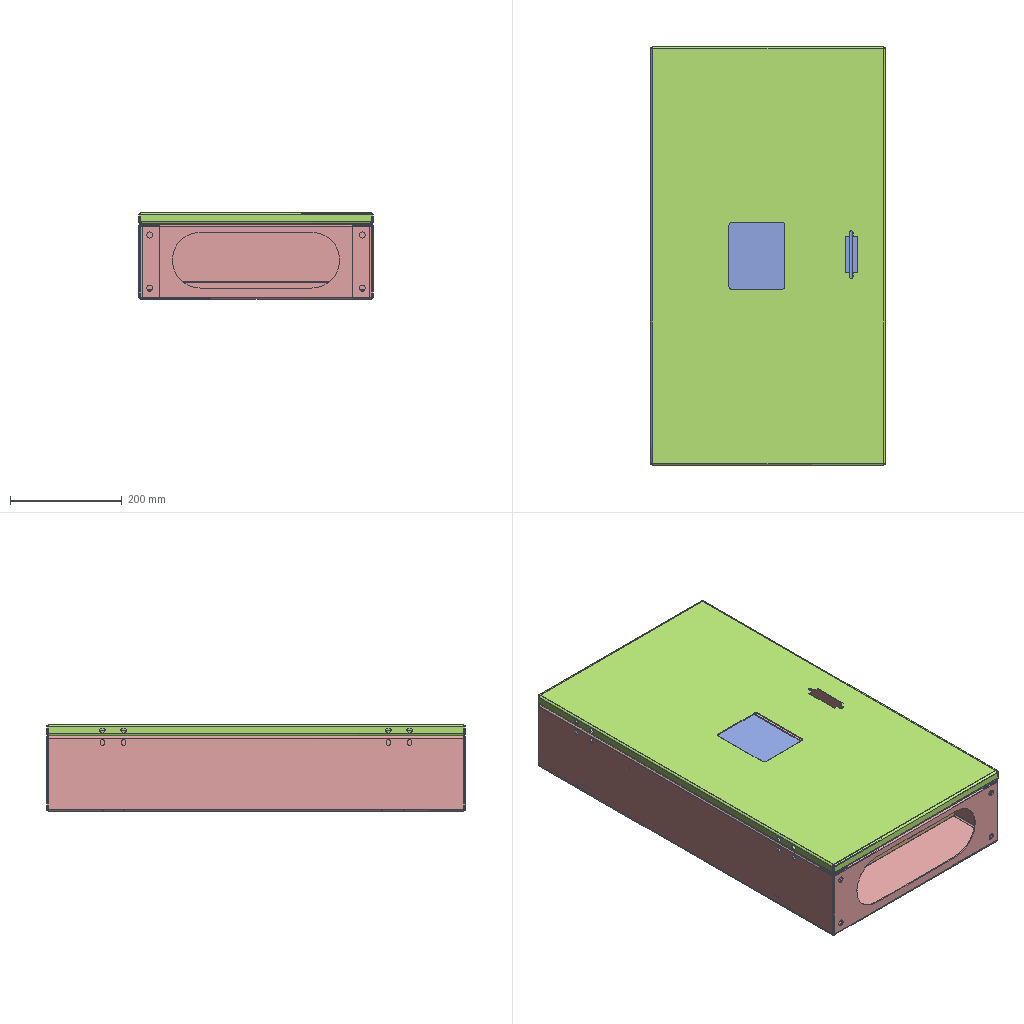Assembly | SolidWorks | 6 different items | 9 placed | box 420 x 750 x 155 mm
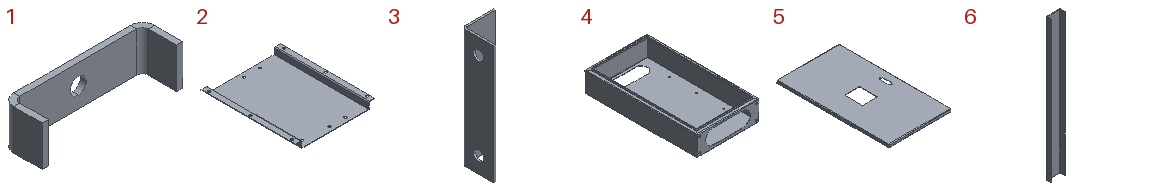Parts list (item | quantity | size | volume | features):
1 | x2 | 35 x 10 x 10 mm | 732.179 mm3 | features FlatPattern 1, ICE 1, SMBaseFlange 1, SheetMetal 1
2 | x1 | 350 x 415 x 30 mm | 330826 mm3 | features EdgeFlange 2, ICE 2, FlatPattern 1, SMBaseFlange 1, SheetMetal 1
3 | x2 | 35 x 35 x 130 mm | 16965 mm3 | features FlatPattern 1, ICE 1, SMBaseFlange 1, SheetMetal 1
4 | x1 | 420 x 750 x 145 mm | 1270936 mm3 | features ICE 5, EdgeFlange 3, FlatPattern 1, SMBaseFlange 1, SheetMetal 1
5 | x1 | 420 x 750 x 20 mm | 745969 mm3 | features ICE 3, EdgeFlange 2, FlatPattern 1, SMBaseFlange 1, SheetMetal 1
6 | x2 | 40 x 15 x 416 mm | 40603 mm3 | features FlatPattern 1, SMBaseFlange 1, SheetMetal 1
Mates (type | each side: item.copy, entity, surface, feature):
Coincident | 4.1 face plane Base-Flange1 | 2.1 face plane Edge-Flange2
Concentric | 4.1 face cylinder Cut-Extrude1 | 2.1 face cylinder Cut-Extrude2 | 2 times
Coincident | 4.1 face plane Edge-Flange14 | 5.1 face plane Edge-Flange2
Coincident | 4.1 face plane Edge-Flange1 | 5.1 face plane Edge-Flange1 | 2 times
Coincident | 4.1 face plane Edge-Flange1 | 3.1 face plane Base-Flange1 | 2 times
Concentric | 4.1 face cylinder Cut-Extrude4 | 3.1 face cylinder Cut-Extrude1
Coincident | 4.1 face plane Edge-Flange1 | 3.2 face plane Base-Flange1 | 2 times
Concentric | 4.1 face cylinder Cut-Extrude4 | 3.2 face cylinder Cut-Extrude1
Coincident | 4.1 face plane Edge-Flange1 | 1.1 face plane Base-Flange1
DistanceDim | 1.1 face plane Base-Flange1 | 4.1 face plane Edge-Flange14
Coincident | 4.1 face plane Edge-Flange1 | 1.2 face plane Base-Flange1
DistanceDim | 1.2 face plane Base-Flange1 | 4.1 face plane Edge-Flange14
DistanceDim | 1.2 face plane Base-Flange1 | 4.1 face plane Edge-Flange1
Coincident | 1.1 face plane Base-Flange1 | 1.2 face plane Base-Flange1
Coincident | 4.1 face plane Base-Flange1 | 6.1 face plane Base-Flange1
Coincident | 4.1 face plane Edge-Flange1 | 6.1 face plane Base-Flange1
Coincident | 4.1 face plane Cut-Extrude2 | 6.1 face plane Base-Flange1
Coincident | 4.1 face plane Base-Flange1 | 6.2 face plane Base-Flange1
Coincident | 4.1 face plane Edge-Flange1 | 6.2 face plane Base-Flange1
DistanceDim | 6.2 face plane Base-Flange1 | 4.1 face plane Edge-Flange1